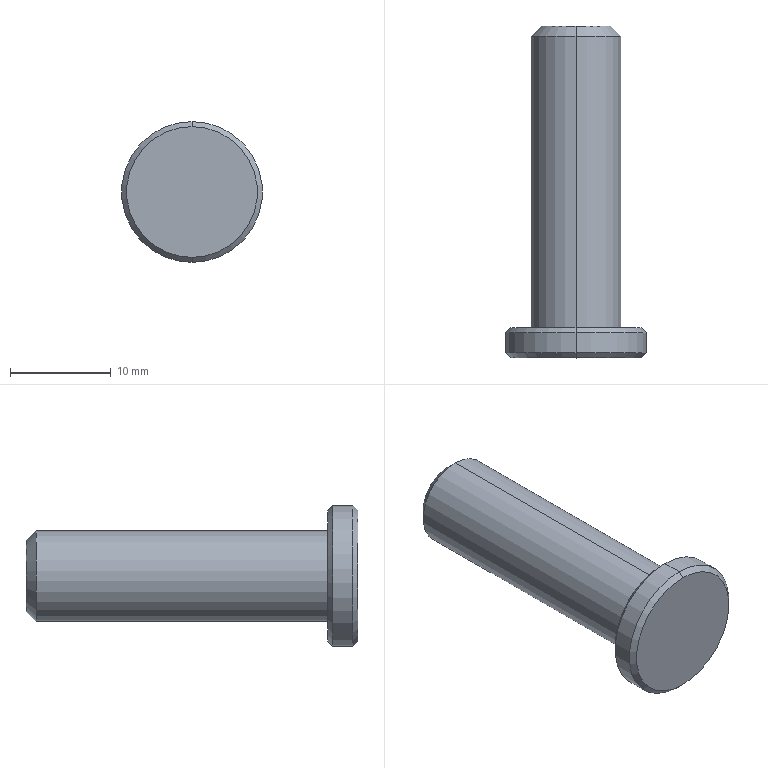Part | SolidWorks | features Chamfer 2, Extrusion 1, ICE 1 | 1 solid | 13 faces | box 14 x 33 x 14 mm | volume 2347 mm3 | cone 6 | cylinder 4 | plane 3 | commonest cylinder face diameters 9 x2 14 x2
STEP:
#1=CARTESIAN_POINT('',(0.,3.,6.5));
#2=VERTEX_POINT('',#1);
#3=CARTESIAN_POINT('',(0.,3.,-6.5));
#4=VERTEX_POINT('',#3);
#5=CARTESIAN_POINT('',(0.,3.,0.));
#6=DIRECTION('',(0.,1.,0.));
#7=DIRECTION('',(0.,0.,1.));
#8=AXIS2_PLACEMENT_3D('',#5,#6,#7);
#9=CIRCLE('',#8,6.5);
#10=EDGE_CURVE('',#2,#4,#9,.T.);
#11=ORIENTED_EDGE('',*,*,#10,.F.);
#12=CARTESIAN_POINT('',(0.,2.5,7.));
#13=VERTEX_POINT('',#12);
#14=CARTESIAN_POINT('',(0.,3.,6.5));
#15=DIRECTION('',(0.,-0.7071,0.7071));
#16=VECTOR('',#15,1000.);
#17=LINE('',#14,#16);
#18=EDGE_CURVE('',#2,#13,#17,.T.);
#19=ORIENTED_EDGE('',*,*,#18,.T.);
#20=CARTESIAN_POINT('',(0.,2.5,-7.));
#21=VERTEX_POINT('',#20);
#22=CARTESIAN_POINT('',(0.,2.5,0.));
#23=DIRECTION('',(0.,-1.,0.));
#24=DIRECTION('',(0.,0.,1.));
#25=AXIS2_PLACEMENT_3D('',#22,#23,#24);
#26=CIRCLE('',#25,7.);
#27=EDGE_CURVE('',#21,#13,#26,.T.);
#28=ORIENTED_EDGE('',*,*,#27,.F.);
#29=CARTESIAN_POINT('',(0.,3.,-6.5));
#30=DIRECTION('',(0.,-0.7071,-0.7071));
#31=VECTOR('',#30,1000.);
#32=LINE('',#29,#31);
#33=EDGE_CURVE('',#4,#21,#32,.T.);
#34=ORIENTED_EDGE('',*,*,#33,.F.);
#35=EDGE_LOOP('',(#11,#19,#28,#34));
#36=FACE_OUTER_BOUND('',#35,.T.);
#37=CARTESIAN_POINT('',(0.,3.,0.));
#38=DIRECTION('',(0.,-1.,0.));
#39=DIRECTION('',(0.,0.,-1.));
#40=AXIS2_PLACEMENT_3D('',#37,#38,#39);
#41=CONICAL_SURFACE('',#40,6.5,0.7854);
#42=ADVANCED_FACE('',(#36),#41,.T.);
#43=CARTESIAN_POINT('',(0.,0.,-6.5));
#44=VERTEX_POINT('',#43);
#45=CARTESIAN_POINT('',(0.,0.,6.5));
#46=VERTEX_POINT('',#45);
#47=CARTESIAN_POINT('',(0.,0.,0.));
#48=DIRECTION('',(0.,-1.,0.));
#49=DIRECTION('',(0.,0.,1.));
#50=AXIS2_PLACEMENT_3D('',#47,#48,#49);
#51=CIRCLE('',#50,6.5);
#52=EDGE_CURVE('',#44,#46,#51,.T.);
#53=ORIENTED_EDGE('',*,*,#52,.F.);
#54=CARTESIAN_POINT('',(0.,0.5,-7.));
#55=VERTEX_POINT('',#54);
#56=CARTESIAN_POINT('',(0.,0.5,-7.));
#57=DIRECTION('',(0.,0.7071,-0.7071));
#58=VECTOR('',#57,1000.);
#59=LINE('',#56,#58);
#60=EDGE_CURVE('',#44,#55,#59,.T.);
#61=ORIENTED_EDGE('',*,*,#60,.T.);
#62=CARTESIAN_POINT('',(0.,0.5,7.));
#63=VERTEX_POINT('',#62);
#64=CARTESIAN_POINT('',(0.,0.5,0.));
#65=DIRECTION('',(0.,1.,0.));
#66=DIRECTION('',(0.,0.,1.));
#67=AXIS2_PLACEMENT_3D('',#64,#65,#66);
#68=CIRCLE('',#67,7.);
#69=EDGE_CURVE('',#63,#55,#68,.T.);
#70=ORIENTED_EDGE('',*,*,#69,.F.);
#71=CARTESIAN_POINT('',(0.,0.5,7.));
#72=DIRECTION('',(0.,0.7071,0.7071));
#73=VECTOR('',#72,1000.);
#74=LINE('',#71,#73);
#75=EDGE_CURVE('',#46,#63,#74,.T.);
#76=ORIENTED_EDGE('',*,*,#75,.F.);
#77=EDGE_LOOP('',(#53,#61,#70,#76));
#78=FACE_OUTER_BOUND('',#77,.T.);
#79=CARTESIAN_POINT('',(0.,0.5,0.));
#80=DIRECTION('',(0.,1.,0.));
#81=DIRECTION('',(0.,0.,1.));
#82=AXIS2_PLACEMENT_3D('',#79,#80,#81);
#83=CONICAL_SURFACE('',#82,7.,0.7854);
#84=ADVANCED_FACE('',(#78),#83,.T.);
#85=CARTESIAN_POINT('',(0.,33.,3.5));
#86=VERTEX_POINT('',#85);
#87=CARTESIAN_POINT('',(0.,33.,-3.5));
#88=VERTEX_POINT('',#87);
#89=CARTESIAN_POINT('',(0.,33.,0.));
#90=DIRECTION('',(0.,1.,0.));
#91=DIRECTION('',(0.,0.,1.));
#92=AXIS2_PLACEMENT_3D('',#89,#90,#91);
#93=CIRCLE('',#92,3.5);
#94=EDGE_CURVE('',#86,#88,#93,.T.);
#95=ORIENTED_EDGE('',*,*,#94,.F.);
#96=CARTESIAN_POINT('',(0.,32.,4.5));
#97=VERTEX_POINT('',#96);
#98=CARTESIAN_POINT('',(0.,33.,3.5));
#99=DIRECTION('',(0.,-0.7071,0.7071));
#100=VECTOR('',#99,1000.);
#101=LINE('',#98,#100);
#102=EDGE_CURVE('',#86,#97,#101,.T.);
#103=ORIENTED_EDGE('',*,*,#102,.T.);
#104=CARTESIAN_POINT('',(0.,32.,-4.5));
#105=VERTEX_POINT('',#104);
#106=CARTESIAN_POINT('',(0.,32.,0.));
#107=DIRECTION('',(0.,-1.,0.));
#108=DIRECTION('',(0.,0.,1.));
#109=AXIS2_PLACEMENT_3D('',#106,#107,#108);
#110=CIRCLE('',#109,4.5);
#111=EDGE_CURVE('',#105,#97,#110,.T.);
#112=ORIENTED_EDGE('',*,*,#111,.F.);
#113=CARTESIAN_POINT('',(0.,33.,-3.5));
#114=DIRECTION('',(0.,-0.7071,-0.7071));
#115=VECTOR('',#114,1000.);
#116=LINE('',#113,#115);
#117=EDGE_CURVE('',#88,#105,#116,.T.);
#118=ORIENTED_EDGE('',*,*,#117,.F.);
#119=EDGE_LOOP('',(#95,#103,#112,#118));
#120=FACE_OUTER_BOUND('',#119,.T.);
#121=CARTESIAN_POINT('',(0.,33.,0.));
#122=DIRECTION('',(0.,-1.,0.));
#123=DIRECTION('',(0.,0.,-1.));
#124=AXIS2_PLACEMENT_3D('',#121,#122,#123);
#125=CONICAL_SURFACE('',#124,3.5,0.7854);
#126=ADVANCED_FACE('',(#120),#125,.T.);
#127=ORIENTED_EDGE('',*,*,#111,.T.);
#128=CARTESIAN_POINT('',(0.,3.,4.5));
#129=VERTEX_POINT('',#128);
#130=CARTESIAN_POINT('',(0.,33.,4.5));
#131=DIRECTION('',(0.,-1.,0.));
#132=VECTOR('',#131,1000.);
#133=LINE('',#130,#132);
#134=EDGE_CURVE('',#97,#129,#133,.T.);
#135=ORIENTED_EDGE('',*,*,#134,.T.);
#136=CARTESIAN_POINT('',(0.,3.,-4.5));
#137=VERTEX_POINT('',#136);
#138=CARTESIAN_POINT('',(0.,3.,0.));
#139=DIRECTION('',(0.,1.,0.));
#140=DIRECTION('',(0.,0.,1.));
#141=AXIS2_PLACEMENT_3D('',#138,#139,#140);
#142=CIRCLE('',#141,4.5);
#143=EDGE_CURVE('',#129,#137,#142,.T.);
#144=ORIENTED_EDGE('',*,*,#143,.T.);
#145=CARTESIAN_POINT('',(0.,33.,-4.5));
#146=DIRECTION('',(0.,-1.,0.));
#147=VECTOR('',#146,1000.);
#148=LINE('',#145,#147);
#149=EDGE_CURVE('',#105,#137,#148,.T.);
#150=ORIENTED_EDGE('',*,*,#149,.F.);
#151=EDGE_LOOP('',(#127,#135,#144,#150));
#152=FACE_OUTER_BOUND('',#151,.T.);
#153=CARTESIAN_POINT('',(0.,33.,0.));
#154=DIRECTION('',(0.,-1.,0.));
#155=DIRECTION('',(0.,0.,-1.));
#156=AXIS2_PLACEMENT_3D('',#153,#154,#155);
#157=CYLINDRICAL_SURFACE('',#156,4.5);
#158=ADVANCED_FACE('',(#152),#157,.T.);
#159=ORIENTED_EDGE('',*,*,#27,.T.);
#160=CARTESIAN_POINT('',(0.,3.,7.));
#161=DIRECTION('',(0.,-1.,0.));
#162=VECTOR('',#161,1000.);
#163=LINE('',#160,#162);
#164=EDGE_CURVE('',#13,#63,#163,.T.);
#165=ORIENTED_EDGE('',*,*,#164,.T.);
#166=ORIENTED_EDGE('',*,*,#69,.T.);
#167=CARTESIAN_POINT('',(0.,3.,-7.));
#168=DIRECTION('',(0.,-1.,0.));
#169=VECTOR('',#168,1000.);
#170=LINE('',#167,#169);
#171=EDGE_CURVE('',#21,#55,#170,.T.);
#172=ORIENTED_EDGE('',*,*,#171,.F.);
#173=EDGE_LOOP('',(#159,#165,#166,#172));
#174=FACE_OUTER_BOUND('',#173,.T.);
#175=CARTESIAN_POINT('',(0.,3.,0.));
#176=DIRECTION('',(0.,-1.,0.));
#177=DIRECTION('',(0.,0.,-1.));
#178=AXIS2_PLACEMENT_3D('',#175,#176,#177);
#179=CYLINDRICAL_SURFACE('',#178,7.);
#180=ADVANCED_FACE('',(#174),#179,.T.);
#181=ORIENTED_EDGE('',*,*,#164,.F.);
#182=CARTESIAN_POINT('',(0.,2.5,0.));
#183=DIRECTION('',(0.,-1.,0.));
#184=DIRECTION('',(0.,0.,1.));
#185=AXIS2_PLACEMENT_3D('',#182,#183,#184);
#186=CIRCLE('',#185,7.);
#187=EDGE_CURVE('',#13,#21,#186,.T.);
#188=ORIENTED_EDGE('',*,*,#187,.T.);
#189=ORIENTED_EDGE('',*,*,#171,.T.);
#190=CARTESIAN_POINT('',(0.,0.5,0.));
#191=DIRECTION('',(0.,1.,0.));
#192=DIRECTION('',(0.,0.,1.));
#193=AXIS2_PLACEMENT_3D('',#190,#191,#192);
#194=CIRCLE('',#193,7.);
#195=EDGE_CURVE('',#55,#63,#194,.T.);
#196=ORIENTED_EDGE('',*,*,#195,.T.);
#197=EDGE_LOOP('',(#181,#188,#189,#196));
#198=FACE_OUTER_BOUND('',#197,.T.);
#199=CARTESIAN_POINT('',(0.,3.,0.));
#200=DIRECTION('',(0.,-1.,0.));
#201=DIRECTION('',(0.,0.,-1.));
#202=AXIS2_PLACEMENT_3D('',#199,#200,#201);
#203=CYLINDRICAL_SURFACE('',#202,7.);
#204=ADVANCED_FACE('',(#198),#203,.T.);
#205=CARTESIAN_POINT('',(0.,3.,0.));
#206=DIRECTION('',(0.,1.,0.));
#207=DIRECTION('',(0.,0.,1.));
#208=AXIS2_PLACEMENT_3D('',#205,#206,#207);
#209=CIRCLE('',#208,6.5);
#210=EDGE_CURVE('',#4,#2,#209,.T.);
#211=ORIENTED_EDGE('',*,*,#210,.T.);
#212=ORIENTED_EDGE('',*,*,#10,.T.);
#213=EDGE_LOOP('',(#211,#212));
#214=FACE_OUTER_BOUND('',#213,.T.);
#215=CARTESIAN_POINT('',(0.,3.,0.));
#216=DIRECTION('',(0.,1.,0.));
#217=DIRECTION('',(0.,0.,1.));
#218=AXIS2_PLACEMENT_3D('',#215,#216,#217);
#219=CIRCLE('',#218,4.5);
#220=EDGE_CURVE('',#137,#129,#219,.T.);
#221=ORIENTED_EDGE('',*,*,#220,.F.);
#222=ORIENTED_EDGE('',*,*,#143,.F.);
#223=EDGE_LOOP('',(#221,#222));
#224=FACE_BOUND('',#223,.T.);
#225=CARTESIAN_POINT('',(0.,3.,0.));
#226=DIRECTION('',(0.,1.,0.));
#227=DIRECTION('',(0.,0.,1.));
#228=AXIS2_PLACEMENT_3D('',#225,#226,#227);
#229=PLANE('',#228);
#230=ADVANCED_FACE('',(#214,#224),#229,.T.);
#231=CARTESIAN_POINT('',(0.,0.,0.));
#232=DIRECTION('',(0.,-1.,0.));
#233=DIRECTION('',(0.,0.,1.));
#234=AXIS2_PLACEMENT_3D('',#231,#232,#233);
#235=CIRCLE('',#234,6.5);
#236=EDGE_CURVE('',#46,#44,#235,.T.);
#237=ORIENTED_EDGE('',*,*,#236,.T.);
#238=ORIENTED_EDGE('',*,*,#52,.T.);
#239=EDGE_LOOP('',(#237,#238));
#240=FACE_OUTER_BOUND('',#239,.T.);
#241=CARTESIAN_POINT('',(0.,0.,0.));
#242=DIRECTION('',(0.,1.,0.));
#243=DIRECTION('',(0.,0.,1.));
#244=AXIS2_PLACEMENT_3D('',#241,#242,#243);
#245=PLANE('',#244);
#246=ADVANCED_FACE('',(#240),#245,.F.);
#247=ORIENTED_EDGE('',*,*,#134,.F.);
#248=CARTESIAN_POINT('',(0.,32.,0.));
#249=DIRECTION('',(0.,-1.,0.));
#250=DIRECTION('',(0.,0.,1.));
#251=AXIS2_PLACEMENT_3D('',#248,#249,#250);
#252=CIRCLE('',#251,4.5);
#253=EDGE_CURVE('',#97,#105,#252,.T.);
#254=ORIENTED_EDGE('',*,*,#253,.T.);
#255=ORIENTED_EDGE('',*,*,#149,.T.);
#256=ORIENTED_EDGE('',*,*,#220,.T.);
#257=EDGE_LOOP('',(#247,#254,#255,#256));
#258=FACE_OUTER_BOUND('',#257,.T.);
#259=CARTESIAN_POINT('',(0.,33.,0.));
#260=DIRECTION('',(0.,-1.,0.));
#261=DIRECTION('',(0.,0.,-1.));
#262=AXIS2_PLACEMENT_3D('',#259,#260,#261);
#263=CYLINDRICAL_SURFACE('',#262,4.5);
#264=ADVANCED_FACE('',(#258),#263,.T.);
#265=CARTESIAN_POINT('',(0.,33.,0.));
#266=DIRECTION('',(0.,1.,0.));
#267=DIRECTION('',(0.,0.,1.));
#268=AXIS2_PLACEMENT_3D('',#265,#266,#267);
#269=CIRCLE('',#268,3.5);
#270=EDGE_CURVE('',#88,#86,#269,.T.);
#271=ORIENTED_EDGE('',*,*,#270,.T.);
#272=ORIENTED_EDGE('',*,*,#94,.T.);
#273=EDGE_LOOP('',(#271,#272));
#274=FACE_OUTER_BOUND('',#273,.T.);
#275=CARTESIAN_POINT('',(0.,33.,0.));
#276=DIRECTION('',(0.,1.,0.));
#277=DIRECTION('',(0.,0.,1.));
#278=AXIS2_PLACEMENT_3D('',#275,#276,#277);
#279=PLANE('',#278);
#280=ADVANCED_FACE('',(#274),#279,.T.);
#281=ORIENTED_EDGE('',*,*,#102,.F.);
#282=ORIENTED_EDGE('',*,*,#270,.F.);
#283=ORIENTED_EDGE('',*,*,#117,.T.);
#284=ORIENTED_EDGE('',*,*,#253,.F.);
#285=EDGE_LOOP('',(#281,#282,#283,#284));
#286=FACE_OUTER_BOUND('',#285,.T.);
#287=CARTESIAN_POINT('',(0.,33.,0.));
#288=DIRECTION('',(0.,-1.,0.));
#289=DIRECTION('',(0.,0.,-1.));
#290=AXIS2_PLACEMENT_3D('',#287,#288,#289);
#291=CONICAL_SURFACE('',#290,3.5,0.7854);
#292=ADVANCED_FACE('',(#286),#291,.T.);
#293=ORIENTED_EDGE('',*,*,#60,.F.);
#294=ORIENTED_EDGE('',*,*,#236,.F.);
#295=ORIENTED_EDGE('',*,*,#75,.T.);
#296=ORIENTED_EDGE('',*,*,#195,.F.);
#297=EDGE_LOOP('',(#293,#294,#295,#296));
#298=FACE_OUTER_BOUND('',#297,.T.);
#299=CARTESIAN_POINT('',(0.,0.5,0.));
#300=DIRECTION('',(0.,1.,0.));
#301=DIRECTION('',(0.,0.,1.));
#302=AXIS2_PLACEMENT_3D('',#299,#300,#301);
#303=CONICAL_SURFACE('',#302,7.,0.7854);
#304=ADVANCED_FACE('',(#298),#303,.T.);
#305=ORIENTED_EDGE('',*,*,#18,.F.);
#306=ORIENTED_EDGE('',*,*,#210,.F.);
#307=ORIENTED_EDGE('',*,*,#33,.T.);
#308=ORIENTED_EDGE('',*,*,#187,.F.);
#309=EDGE_LOOP('',(#305,#306,#307,#308));
#310=FACE_OUTER_BOUND('',#309,.T.);
#311=CARTESIAN_POINT('',(0.,3.,0.));
#312=DIRECTION('',(0.,-1.,0.));
#313=DIRECTION('',(0.,0.,-1.));
#314=AXIS2_PLACEMENT_3D('',#311,#312,#313);
#315=CONICAL_SURFACE('',#314,6.5,0.7854);
#316=ADVANCED_FACE('',(#310),#315,.T.);
#317=CLOSED_SHELL('',(#42,#84,#126,#158,#180,#204,#230,#246,#264,#280,#292,#304,#316));
#318=MANIFOLD_SOLID_BREP('',#317);
#319=CARTESIAN_POINT('',(0.,0.,0.));
#320=DIRECTION('',(0.,0.,1.));
#321=DIRECTION('',(1.,0.,0.));
#322=AXIS2_PLACEMENT_3D('',#319,#320,#321);
#323=(LENGTH_UNIT()NAMED_UNIT(*)SI_UNIT(.MILLI.,.METRE.));
#324=UNCERTAINTY_MEASURE_WITH_UNIT(LENGTH_MEASURE(0.00001),#323,'','');
#325=(NAMED_UNIT(*)PLANE_ANGLE_UNIT()SI_UNIT($,.RADIAN.));
#326=(NAMED_UNIT(*)SI_UNIT($,.STERADIAN.)SOLID_ANGLE_UNIT());
#327=(GEOMETRIC_REPRESENTATION_CONTEXT(3)GLOBAL_UNCERTAINTY_ASSIGNED_CONTEXT((#324))GLOBAL_UNIT_ASSIGNED_CONTEXT((#323,#325,#326))REPRESENTATION_CONTEXT('',''));
#328=ADVANCED_BREP_SHAPE_REPRESENTATION('',(#318,#322),#327);